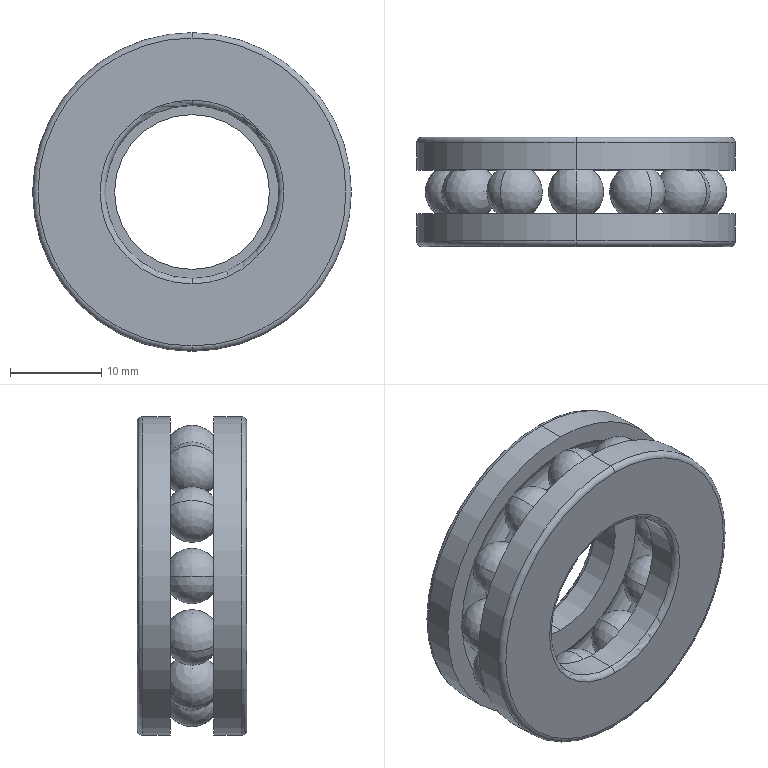Part | SolidWorks | features BaseBody 1 | 1 solid | 70 faces | box 35 x 12 x 35 mm | volume 6237 mm3 | torus 32 | sphere 24 | cylinder 8 | plane 6 | commonest cylinder face diameters 35 x4 17 x2 19 x2